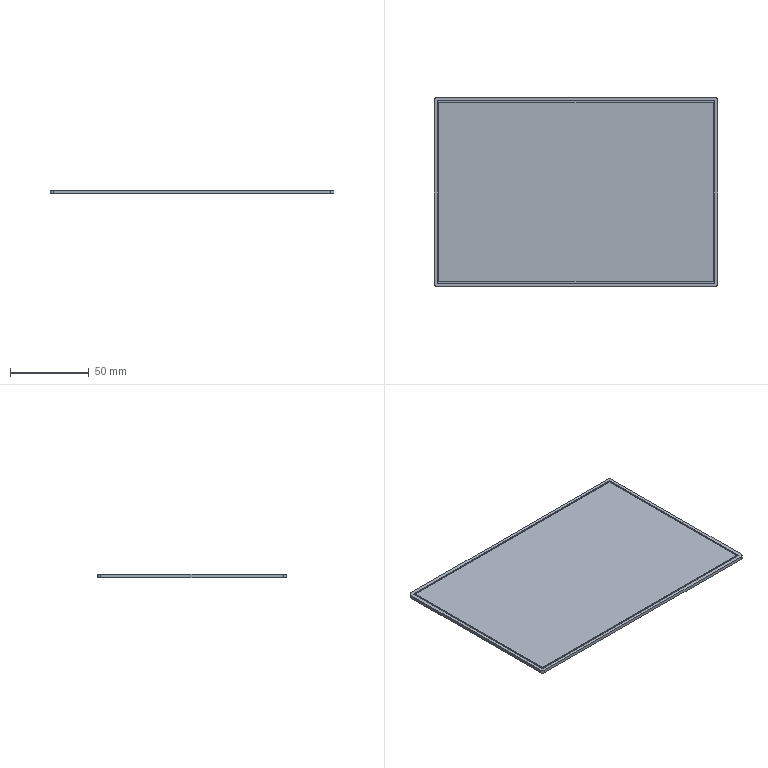Part | SolidWorks | features Extrusion 1, ICE 1 | 1 solid | 20 faces | box 180 x 120 x 2 mm | volume 42903 mm3 | plane 16 | cylinder 4 | commonest cylinder face diameters 4 x4
STEP:
#1=CARTESIAN_POINT('',(90.,58.,0.));
#2=VERTEX_POINT('',#1);
#3=CARTESIAN_POINT('',(88.,60.,0.));
#4=VERTEX_POINT('',#3);
#5=CARTESIAN_POINT('',(88.,58.,0.));
#6=DIRECTION('',(0.,0.,1.));
#7=DIRECTION('',(-1.,0.,0.));
#8=AXIS2_PLACEMENT_3D('',#5,#6,#7);
#9=CIRCLE('',#8,2.);
#10=EDGE_CURVE('',#2,#4,#9,.T.);
#11=ORIENTED_EDGE('',*,*,#10,.T.);
#12=CARTESIAN_POINT('',(88.,60.,2.));
#13=VERTEX_POINT('',#12);
#14=CARTESIAN_POINT('',(88.,60.,2.));
#15=DIRECTION('',(0.,0.,-1.));
#16=VECTOR('',#15,1000.);
#17=LINE('',#14,#16);
#18=EDGE_CURVE('',#13,#4,#17,.T.);
#19=ORIENTED_EDGE('',*,*,#18,.F.);
#20=CARTESIAN_POINT('',(90.,58.,2.));
#21=VERTEX_POINT('',#20);
#22=CARTESIAN_POINT('',(88.,58.,2.));
#23=DIRECTION('',(0.,0.,1.));
#24=DIRECTION('',(-1.,0.,0.));
#25=AXIS2_PLACEMENT_3D('',#22,#23,#24);
#26=CIRCLE('',#25,2.);
#27=EDGE_CURVE('',#21,#13,#26,.T.);
#28=ORIENTED_EDGE('',*,*,#27,.F.);
#29=CARTESIAN_POINT('',(90.,58.,2.));
#30=DIRECTION('',(0.,0.,-1.));
#31=VECTOR('',#30,1000.);
#32=LINE('',#29,#31);
#33=EDGE_CURVE('',#21,#2,#32,.T.);
#34=ORIENTED_EDGE('',*,*,#33,.T.);
#35=EDGE_LOOP('',(#11,#19,#28,#34));
#36=FACE_OUTER_BOUND('',#35,.T.);
#37=CARTESIAN_POINT('',(88.,58.,2.));
#38=DIRECTION('',(0.,0.,-1.));
#39=DIRECTION('',(-1.,0.,0.));
#40=AXIS2_PLACEMENT_3D('',#37,#38,#39);
#41=CYLINDRICAL_SURFACE('',#40,2.);
#42=ADVANCED_FACE('',(#36),#41,.T.);
#43=CARTESIAN_POINT('',(-88.,60.,0.));
#44=VERTEX_POINT('',#43);
#45=CARTESIAN_POINT('',(88.,60.,0.));
#46=DIRECTION('',(-1.,0.,0.));
#47=VECTOR('',#46,1000.);
#48=LINE('',#45,#47);
#49=EDGE_CURVE('',#4,#44,#48,.T.);
#50=ORIENTED_EDGE('',*,*,#49,.T.);
#51=CARTESIAN_POINT('',(-88.,60.,2.));
#52=VERTEX_POINT('',#51);
#53=CARTESIAN_POINT('',(-88.,60.,2.));
#54=DIRECTION('',(0.,0.,-1.));
#55=VECTOR('',#54,1000.);
#56=LINE('',#53,#55);
#57=EDGE_CURVE('',#52,#44,#56,.T.);
#58=ORIENTED_EDGE('',*,*,#57,.F.);
#59=CARTESIAN_POINT('',(88.,60.,2.));
#60=DIRECTION('',(-1.,0.,0.));
#61=VECTOR('',#60,1000.);
#62=LINE('',#59,#61);
#63=EDGE_CURVE('',#13,#52,#62,.T.);
#64=ORIENTED_EDGE('',*,*,#63,.F.);
#65=ORIENTED_EDGE('',*,*,#18,.T.);
#66=EDGE_LOOP('',(#50,#58,#64,#65));
#67=FACE_OUTER_BOUND('',#66,.T.);
#68=CARTESIAN_POINT('',(88.,60.,2.));
#69=DIRECTION('',(0.,-1.,0.));
#70=DIRECTION('',(1.,0.,0.));
#71=AXIS2_PLACEMENT_3D('',#68,#69,#70);
#72=PLANE('',#71);
#73=ADVANCED_FACE('',(#67),#72,.F.);
#74=CARTESIAN_POINT('',(-90.,58.,0.));
#75=VERTEX_POINT('',#74);
#76=CARTESIAN_POINT('',(-88.,58.,0.));
#77=DIRECTION('',(0.,0.,1.));
#78=DIRECTION('',(1.,0.,0.));
#79=AXIS2_PLACEMENT_3D('',#76,#77,#78);
#80=CIRCLE('',#79,2.);
#81=EDGE_CURVE('',#44,#75,#80,.T.);
#82=ORIENTED_EDGE('',*,*,#81,.T.);
#83=CARTESIAN_POINT('',(-90.,58.,2.));
#84=VERTEX_POINT('',#83);
#85=CARTESIAN_POINT('',(-90.,58.,2.));
#86=DIRECTION('',(0.,0.,-1.));
#87=VECTOR('',#86,1000.);
#88=LINE('',#85,#87);
#89=EDGE_CURVE('',#84,#75,#88,.T.);
#90=ORIENTED_EDGE('',*,*,#89,.F.);
#91=CARTESIAN_POINT('',(-88.,58.,2.));
#92=DIRECTION('',(0.,0.,1.));
#93=DIRECTION('',(1.,0.,0.));
#94=AXIS2_PLACEMENT_3D('',#91,#92,#93);
#95=CIRCLE('',#94,2.);
#96=EDGE_CURVE('',#52,#84,#95,.T.);
#97=ORIENTED_EDGE('',*,*,#96,.F.);
#98=ORIENTED_EDGE('',*,*,#57,.T.);
#99=EDGE_LOOP('',(#82,#90,#97,#98));
#100=FACE_OUTER_BOUND('',#99,.T.);
#101=CARTESIAN_POINT('',(-88.,58.,2.));
#102=DIRECTION('',(0.,0.,-1.));
#103=DIRECTION('',(-1.,0.,0.));
#104=AXIS2_PLACEMENT_3D('',#101,#102,#103);
#105=CYLINDRICAL_SURFACE('',#104,2.);
#106=ADVANCED_FACE('',(#100),#105,.T.);
#107=CARTESIAN_POINT('',(-90.,-58.,0.));
#108=VERTEX_POINT('',#107);
#109=CARTESIAN_POINT('',(-90.,58.,0.));
#110=DIRECTION('',(0.,-1.,0.));
#111=VECTOR('',#110,1000.);
#112=LINE('',#109,#111);
#113=EDGE_CURVE('',#75,#108,#112,.T.);
#114=ORIENTED_EDGE('',*,*,#113,.T.);
#115=CARTESIAN_POINT('',(-90.,-58.,2.));
#116=VERTEX_POINT('',#115);
#117=CARTESIAN_POINT('',(-90.,-58.,2.));
#118=DIRECTION('',(0.,0.,-1.));
#119=VECTOR('',#118,1000.);
#120=LINE('',#117,#119);
#121=EDGE_CURVE('',#116,#108,#120,.T.);
#122=ORIENTED_EDGE('',*,*,#121,.F.);
#123=CARTESIAN_POINT('',(-90.,58.,2.));
#124=DIRECTION('',(0.,-1.,0.));
#125=VECTOR('',#124,1000.);
#126=LINE('',#123,#125);
#127=EDGE_CURVE('',#84,#116,#126,.T.);
#128=ORIENTED_EDGE('',*,*,#127,.F.);
#129=ORIENTED_EDGE('',*,*,#89,.T.);
#130=EDGE_LOOP('',(#114,#122,#128,#129));
#131=FACE_OUTER_BOUND('',#130,.T.);
#132=CARTESIAN_POINT('',(-90.,58.,2.));
#133=DIRECTION('',(1.,0.,0.));
#134=DIRECTION('',(0.,1.,0.));
#135=AXIS2_PLACEMENT_3D('',#132,#133,#134);
#136=PLANE('',#135);
#137=ADVANCED_FACE('',(#131),#136,.F.);
#138=CARTESIAN_POINT('',(-88.,-60.,0.));
#139=VERTEX_POINT('',#138);
#140=CARTESIAN_POINT('',(-88.,-58.,0.));
#141=DIRECTION('',(0.,0.,1.));
#142=DIRECTION('',(-1.,0.,0.));
#143=AXIS2_PLACEMENT_3D('',#140,#141,#142);
#144=CIRCLE('',#143,2.);
#145=EDGE_CURVE('',#108,#139,#144,.T.);
#146=ORIENTED_EDGE('',*,*,#145,.T.);
#147=CARTESIAN_POINT('',(-88.,-60.,2.));
#148=VERTEX_POINT('',#147);
#149=CARTESIAN_POINT('',(-88.,-60.,2.));
#150=DIRECTION('',(0.,0.,-1.));
#151=VECTOR('',#150,1000.);
#152=LINE('',#149,#151);
#153=EDGE_CURVE('',#148,#139,#152,.T.);
#154=ORIENTED_EDGE('',*,*,#153,.F.);
#155=CARTESIAN_POINT('',(-88.,-58.,2.));
#156=DIRECTION('',(0.,0.,1.));
#157=DIRECTION('',(-1.,0.,0.));
#158=AXIS2_PLACEMENT_3D('',#155,#156,#157);
#159=CIRCLE('',#158,2.);
#160=EDGE_CURVE('',#116,#148,#159,.T.);
#161=ORIENTED_EDGE('',*,*,#160,.F.);
#162=ORIENTED_EDGE('',*,*,#121,.T.);
#163=EDGE_LOOP('',(#146,#154,#161,#162));
#164=FACE_OUTER_BOUND('',#163,.T.);
#165=CARTESIAN_POINT('',(-88.,-58.,2.));
#166=DIRECTION('',(0.,0.,-1.));
#167=DIRECTION('',(-1.,0.,0.));
#168=AXIS2_PLACEMENT_3D('',#165,#166,#167);
#169=CYLINDRICAL_SURFACE('',#168,2.);
#170=ADVANCED_FACE('',(#164),#169,.T.);
#171=CARTESIAN_POINT('',(88.,-60.,0.));
#172=VERTEX_POINT('',#171);
#173=CARTESIAN_POINT('',(88.,-60.,0.));
#174=DIRECTION('',(1.,0.,0.));
#175=VECTOR('',#174,1000.);
#176=LINE('',#173,#175);
#177=EDGE_CURVE('',#139,#172,#176,.T.);
#178=ORIENTED_EDGE('',*,*,#177,.T.);
#179=CARTESIAN_POINT('',(88.,-60.,2.));
#180=VERTEX_POINT('',#179);
#181=CARTESIAN_POINT('',(88.,-60.,2.));
#182=DIRECTION('',(0.,0.,-1.));
#183=VECTOR('',#182,1000.);
#184=LINE('',#181,#183);
#185=EDGE_CURVE('',#180,#172,#184,.T.);
#186=ORIENTED_EDGE('',*,*,#185,.F.);
#187=CARTESIAN_POINT('',(88.,-60.,2.));
#188=DIRECTION('',(1.,0.,0.));
#189=VECTOR('',#188,1000.);
#190=LINE('',#187,#189);
#191=EDGE_CURVE('',#148,#180,#190,.T.);
#192=ORIENTED_EDGE('',*,*,#191,.F.);
#193=ORIENTED_EDGE('',*,*,#153,.T.);
#194=EDGE_LOOP('',(#178,#186,#192,#193));
#195=FACE_OUTER_BOUND('',#194,.T.);
#196=CARTESIAN_POINT('',(88.,-60.,2.));
#197=DIRECTION('',(0.,1.,0.));
#198=DIRECTION('',(-1.,0.,0.));
#199=AXIS2_PLACEMENT_3D('',#196,#197,#198);
#200=PLANE('',#199);
#201=ADVANCED_FACE('',(#195),#200,.F.);
#202=CARTESIAN_POINT('',(90.,-58.,0.));
#203=VERTEX_POINT('',#202);
#204=CARTESIAN_POINT('',(88.,-58.,0.));
#205=DIRECTION('',(0.,0.,1.));
#206=DIRECTION('',(-1.,0.,0.));
#207=AXIS2_PLACEMENT_3D('',#204,#205,#206);
#208=CIRCLE('',#207,2.);
#209=EDGE_CURVE('',#172,#203,#208,.T.);
#210=ORIENTED_EDGE('',*,*,#209,.T.);
#211=CARTESIAN_POINT('',(90.,-58.,2.));
#212=VERTEX_POINT('',#211);
#213=CARTESIAN_POINT('',(90.,-58.,2.));
#214=DIRECTION('',(0.,0.,-1.));
#215=VECTOR('',#214,1000.);
#216=LINE('',#213,#215);
#217=EDGE_CURVE('',#212,#203,#216,.T.);
#218=ORIENTED_EDGE('',*,*,#217,.F.);
#219=CARTESIAN_POINT('',(88.,-58.,2.));
#220=DIRECTION('',(0.,0.,1.));
#221=DIRECTION('',(-1.,0.,0.));
#222=AXIS2_PLACEMENT_3D('',#219,#220,#221);
#223=CIRCLE('',#222,2.);
#224=EDGE_CURVE('',#180,#212,#223,.T.);
#225=ORIENTED_EDGE('',*,*,#224,.F.);
#226=ORIENTED_EDGE('',*,*,#185,.T.);
#227=EDGE_LOOP('',(#210,#218,#225,#226));
#228=FACE_OUTER_BOUND('',#227,.T.);
#229=CARTESIAN_POINT('',(88.,-58.,2.));
#230=DIRECTION('',(0.,0.,-1.));
#231=DIRECTION('',(-1.,0.,0.));
#232=AXIS2_PLACEMENT_3D('',#229,#230,#231);
#233=CYLINDRICAL_SURFACE('',#232,2.);
#234=ADVANCED_FACE('',(#228),#233,.T.);
#235=CARTESIAN_POINT('',(90.,58.,0.));
#236=DIRECTION('',(0.,1.,0.));
#237=VECTOR('',#236,1000.);
#238=LINE('',#235,#237);
#239=EDGE_CURVE('',#203,#2,#238,.T.);
#240=ORIENTED_EDGE('',*,*,#239,.T.);
#241=ORIENTED_EDGE('',*,*,#33,.F.);
#242=CARTESIAN_POINT('',(90.,58.,2.));
#243=DIRECTION('',(0.,1.,0.));
#244=VECTOR('',#243,1000.);
#245=LINE('',#242,#244);
#246=EDGE_CURVE('',#212,#21,#245,.T.);
#247=ORIENTED_EDGE('',*,*,#246,.F.);
#248=ORIENTED_EDGE('',*,*,#217,.T.);
#249=EDGE_LOOP('',(#240,#241,#247,#248));
#250=FACE_OUTER_BOUND('',#249,.T.);
#251=CARTESIAN_POINT('',(90.,58.,2.));
#252=DIRECTION('',(-1.,0.,0.));
#253=DIRECTION('',(0.,-1.,0.));
#254=AXIS2_PLACEMENT_3D('',#251,#252,#253);
#255=PLANE('',#254);
#256=ADVANCED_FACE('',(#250),#255,.F.);
#257=CARTESIAN_POINT('',(-88.,-58.,2.));
#258=VERTEX_POINT('',#257);
#259=CARTESIAN_POINT('',(88.,-58.,2.));
#260=VERTEX_POINT('',#259);
#261=CARTESIAN_POINT('',(88.,-58.,2.));
#262=DIRECTION('',(1.,0.,0.));
#263=VECTOR('',#262,1000.);
#264=LINE('',#261,#263);
#265=EDGE_CURVE('',#258,#260,#264,.T.);
#266=ORIENTED_EDGE('',*,*,#265,.F.);
#267=CARTESIAN_POINT('',(-88.,58.,2.));
#268=VERTEX_POINT('',#267);
#269=CARTESIAN_POINT('',(-88.,58.,2.));
#270=DIRECTION('',(0.,-1.,0.));
#271=VECTOR('',#270,1000.);
#272=LINE('',#269,#271);
#273=EDGE_CURVE('',#268,#258,#272,.T.);
#274=ORIENTED_EDGE('',*,*,#273,.F.);
#275=CARTESIAN_POINT('',(88.,58.,2.));
#276=VERTEX_POINT('',#275);
#277=CARTESIAN_POINT('',(88.,58.,2.));
#278=DIRECTION('',(-1.,0.,0.));
#279=VECTOR('',#278,1000.);
#280=LINE('',#277,#279);
#281=EDGE_CURVE('',#276,#268,#280,.T.);
#282=ORIENTED_EDGE('',*,*,#281,.F.);
#283=CARTESIAN_POINT('',(88.,58.,2.));
#284=DIRECTION('',(0.,1.,0.));
#285=VECTOR('',#284,1000.);
#286=LINE('',#283,#285);
#287=EDGE_CURVE('',#260,#276,#286,.T.);
#288=ORIENTED_EDGE('',*,*,#287,.F.);
#289=EDGE_LOOP('',(#266,#274,#282,#288));
#290=FACE_BOUND('',#289,.T.);
#291=ORIENTED_EDGE('',*,*,#27,.T.);
#292=ORIENTED_EDGE('',*,*,#63,.T.);
#293=ORIENTED_EDGE('',*,*,#96,.T.);
#294=ORIENTED_EDGE('',*,*,#127,.T.);
#295=ORIENTED_EDGE('',*,*,#160,.T.);
#296=ORIENTED_EDGE('',*,*,#191,.T.);
#297=ORIENTED_EDGE('',*,*,#224,.T.);
#298=ORIENTED_EDGE('',*,*,#246,.T.);
#299=EDGE_LOOP('',(#291,#292,#293,#294,#295,#296,#297,#298));
#300=FACE_OUTER_BOUND('',#299,.T.);
#301=CARTESIAN_POINT('',(88.,58.,2.));
#302=DIRECTION('',(0.,0.,-1.));
#303=DIRECTION('',(-1.,0.,0.));
#304=AXIS2_PLACEMENT_3D('',#301,#302,#303);
#305=PLANE('',#304);
#306=ADVANCED_FACE('',(#290,#300),#305,.F.);
#307=ORIENTED_EDGE('',*,*,#10,.F.);
#308=ORIENTED_EDGE('',*,*,#239,.F.);
#309=ORIENTED_EDGE('',*,*,#209,.F.);
#310=ORIENTED_EDGE('',*,*,#177,.F.);
#311=ORIENTED_EDGE('',*,*,#145,.F.);
#312=ORIENTED_EDGE('',*,*,#113,.F.);
#313=ORIENTED_EDGE('',*,*,#81,.F.);
#314=ORIENTED_EDGE('',*,*,#49,.F.);
#315=EDGE_LOOP('',(#307,#308,#309,#310,#311,#312,#313,#314));
#316=FACE_OUTER_BOUND('',#315,.T.);
#317=CARTESIAN_POINT('',(88.,58.,0.));
#318=DIRECTION('',(0.,0.,-1.));
#319=DIRECTION('',(-1.,0.,0.));
#320=AXIS2_PLACEMENT_3D('',#317,#318,#319);
#321=PLANE('',#320);
#322=ADVANCED_FACE('',(#316),#321,.T.);
#323=ORIENTED_EDGE('',*,*,#273,.T.);
#324=CARTESIAN_POINT('',(-88.,-58.,1.5));
#325=VERTEX_POINT('',#324);
#326=CARTESIAN_POINT('',(-88.,-58.,1.5));
#327=DIRECTION('',(0.,0.,1.));
#328=VECTOR('',#327,1000.);
#329=LINE('',#326,#328);
#330=EDGE_CURVE('',#325,#258,#329,.T.);
#331=ORIENTED_EDGE('',*,*,#330,.F.);
#332=CARTESIAN_POINT('',(-88.,58.,1.5));
#333=VERTEX_POINT('',#332);
#334=CARTESIAN_POINT('',(-88.,58.,1.5));
#335=DIRECTION('',(0.,-1.,0.));
#336=VECTOR('',#335,1000.);
#337=LINE('',#334,#336);
#338=EDGE_CURVE('',#333,#325,#337,.T.);
#339=ORIENTED_EDGE('',*,*,#338,.F.);
#340=CARTESIAN_POINT('',(-88.,58.,1.5));
#341=DIRECTION('',(0.,0.,1.));
#342=VECTOR('',#341,1000.);
#343=LINE('',#340,#342);
#344=EDGE_CURVE('',#333,#268,#343,.T.);
#345=ORIENTED_EDGE('',*,*,#344,.T.);
#346=EDGE_LOOP('',(#323,#331,#339,#345));
#347=FACE_OUTER_BOUND('',#346,.T.);
#348=CARTESIAN_POINT('',(-88.,58.,1.5));
#349=DIRECTION('',(-1.,0.,0.));
#350=DIRECTION('',(0.,0.,1.));
#351=AXIS2_PLACEMENT_3D('',#348,#349,#350);
#352=PLANE('',#351);
#353=ADVANCED_FACE('',(#347),#352,.F.);
#354=ORIENTED_EDGE('',*,*,#281,.T.);
#355=ORIENTED_EDGE('',*,*,#344,.F.);
#356=CARTESIAN_POINT('',(88.,58.,1.5));
#357=VERTEX_POINT('',#356);
#358=CARTESIAN_POINT('',(88.,58.,1.5));
#359=DIRECTION('',(-1.,0.,0.));
#360=VECTOR('',#359,1000.);
#361=LINE('',#358,#360);
#362=EDGE_CURVE('',#357,#333,#361,.T.);
#363=ORIENTED_EDGE('',*,*,#362,.F.);
#364=CARTESIAN_POINT('',(88.,58.,1.5));
#365=DIRECTION('',(0.,0.,1.));
#366=VECTOR('',#365,1000.);
#367=LINE('',#364,#366);
#368=EDGE_CURVE('',#357,#276,#367,.T.);
#369=ORIENTED_EDGE('',*,*,#368,.T.);
#370=EDGE_LOOP('',(#354,#355,#363,#369));
#371=FACE_OUTER_BOUND('',#370,.T.);
#372=CARTESIAN_POINT('',(88.,58.,1.5));
#373=DIRECTION('',(0.,1.,0.));
#374=DIRECTION('',(0.,0.,1.));
#375=AXIS2_PLACEMENT_3D('',#372,#373,#374);
#376=PLANE('',#375);
#377=ADVANCED_FACE('',(#371),#376,.F.);
#378=ORIENTED_EDGE('',*,*,#287,.T.);
#379=ORIENTED_EDGE('',*,*,#368,.F.);
#380=CARTESIAN_POINT('',(88.,-58.,1.5));
#381=VERTEX_POINT('',#380);
#382=CARTESIAN_POINT('',(88.,58.,1.5));
#383=DIRECTION('',(0.,1.,0.));
#384=VECTOR('',#383,1000.);
#385=LINE('',#382,#384);
#386=EDGE_CURVE('',#381,#357,#385,.T.);
#387=ORIENTED_EDGE('',*,*,#386,.F.);
#388=CARTESIAN_POINT('',(88.,-58.,1.5));
#389=DIRECTION('',(0.,0.,1.));
#390=VECTOR('',#389,1000.);
#391=LINE('',#388,#390);
#392=EDGE_CURVE('',#381,#260,#391,.T.);
#393=ORIENTED_EDGE('',*,*,#392,.T.);
#394=EDGE_LOOP('',(#378,#379,#387,#393));
#395=FACE_OUTER_BOUND('',#394,.T.);
#396=CARTESIAN_POINT('',(88.,58.,1.5));
#397=DIRECTION('',(1.,0.,0.));
#398=DIRECTION('',(0.,0.,-1.));
#399=AXIS2_PLACEMENT_3D('',#396,#397,#398);
#400=PLANE('',#399);
#401=ADVANCED_FACE('',(#395),#400,.F.);
#402=ORIENTED_EDGE('',*,*,#265,.T.);
#403=ORIENTED_EDGE('',*,*,#392,.F.);
#404=CARTESIAN_POINT('',(88.,-58.,1.5));
#405=DIRECTION('',(1.,0.,0.));
#406=VECTOR('',#405,1000.);
#407=LINE('',#404,#406);
#408=EDGE_CURVE('',#325,#381,#407,.T.);
#409=ORIENTED_EDGE('',*,*,#408,.F.);
#410=ORIENTED_EDGE('',*,*,#330,.T.);
#411=EDGE_LOOP('',(#402,#403,#409,#410));
#412=FACE_OUTER_BOUND('',#411,.T.);
#413=CARTESIAN_POINT('',(88.,-58.,1.5));
#414=DIRECTION('',(0.,-1.,0.));
#415=DIRECTION('',(0.,0.,-1.));
#416=AXIS2_PLACEMENT_3D('',#413,#414,#415);
#417=PLANE('',#416);
#418=ADVANCED_FACE('',(#412),#417,.F.);
#419=CARTESIAN_POINT('',(87.,-57.,1.5));
#420=VERTEX_POINT('',#419);
#421=CARTESIAN_POINT('',(87.,57.,1.5));
#422=VERTEX_POINT('',#421);
#423=CARTESIAN_POINT('',(87.,57.,1.5));
#424=DIRECTION('',(0.,1.,0.));
#425=VECTOR('',#424,1000.);
#426=LINE('',#423,#425);
#427=EDGE_CURVE('',#420,#422,#426,.T.);
#428=ORIENTED_EDGE('',*,*,#427,.F.);
#429=CARTESIAN_POINT('',(-87.,-57.,1.5));
#430=VERTEX_POINT('',#429);
#431=CARTESIAN_POINT('',(87.,-57.,1.5));
#432=DIRECTION('',(1.,0.,0.));
#433=VECTOR('',#432,1000.);
#434=LINE('',#431,#433);
#435=EDGE_CURVE('',#430,#420,#434,.T.);
#436=ORIENTED_EDGE('',*,*,#435,.F.);
#437=CARTESIAN_POINT('',(-87.,57.,1.5));
#438=VERTEX_POINT('',#437);
#439=CARTESIAN_POINT('',(-87.,57.,1.5));
#440=DIRECTION('',(0.,-1.,0.));
#441=VECTOR('',#440,1000.);
#442=LINE('',#439,#441);
#443=EDGE_CURVE('',#438,#430,#442,.T.);
#444=ORIENTED_EDGE('',*,*,#443,.F.);
#445=CARTESIAN_POINT('',(87.,57.,1.5));
#446=DIRECTION('',(-1.,0.,0.));
#447=VECTOR('',#446,1000.);
#448=LINE('',#445,#447);
#449=EDGE_CURVE('',#422,#438,#448,.T.);
#450=ORIENTED_EDGE('',*,*,#449,.F.);
#451=EDGE_LOOP('',(#428,#436,#444,#450));
#452=FACE_BOUND('',#451,.T.);
#453=ORIENTED_EDGE('',*,*,#338,.T.);
#454=ORIENTED_EDGE('',*,*,#408,.T.);
#455=ORIENTED_EDGE('',*,*,#386,.T.);
#456=ORIENTED_EDGE('',*,*,#362,.T.);
#457=EDGE_LOOP('',(#453,#454,#455,#456));
#458=FACE_OUTER_BOUND('',#457,.T.);
#459=CARTESIAN_POINT('',(0.,0.,1.5));
#460=DIRECTION('',(0.,0.,-1.));
#461=DIRECTION('',(-1.,0.,0.));
#462=AXIS2_PLACEMENT_3D('',#459,#460,#461);
#463=PLANE('',#462);
#464=ADVANCED_FACE('',(#452,#458),#463,.F.);
#465=CARTESIAN_POINT('',(87.,-57.,2.));
#466=VERTEX_POINT('',#465);
#467=CARTESIAN_POINT('',(87.,57.,2.));
#468=VERTEX_POINT('',#467);
#469=CARTESIAN_POINT('',(87.,57.,2.));
#470=DIRECTION('',(0.,1.,0.));
#471=VECTOR('',#470,1000.);
#472=LINE('',#469,#471);
#473=EDGE_CURVE('',#466,#468,#472,.T.);
#474=ORIENTED_EDGE('',*,*,#473,.F.);
#475=CARTESIAN_POINT('',(87.,-57.,1.5));
#476=DIRECTION('',(0.,0.,1.));
#477=VECTOR('',#476,1000.);
#478=LINE('',#475,#477);
#479=EDGE_CURVE('',#420,#466,#478,.T.);
#480=ORIENTED_EDGE('',*,*,#479,.F.);
#481=ORIENTED_EDGE('',*,*,#427,.T.);
#482=CARTESIAN_POINT('',(87.,57.,1.5));
#483=DIRECTION('',(0.,0.,1.));
#484=VECTOR('',#483,1000.);
#485=LINE('',#482,#484);
#486=EDGE_CURVE('',#422,#468,#485,.T.);
#487=ORIENTED_EDGE('',*,*,#486,.T.);
#488=EDGE_LOOP('',(#474,#480,#481,#487));
#489=FACE_OUTER_BOUND('',#488,.T.);
#490=CARTESIAN_POINT('',(87.,57.,1.5));
#491=DIRECTION('',(1.,0.,0.));
#492=DIRECTION('',(0.,0.,-1.));
#493=AXIS2_PLACEMENT_3D('',#490,#491,#492);
#494=PLANE('',#493);
#495=ADVANCED_FACE('',(#489),#494,.T.);
#496=CARTESIAN_POINT('',(-87.,-57.,2.));
#497=VERTEX_POINT('',#496);
#498=CARTESIAN_POINT('',(87.,-57.,2.));
#499=DIRECTION('',(1.,0.,0.));
#500=VECTOR('',#499,1000.);
#501=LINE('',#498,#500);
#502=EDGE_CURVE('',#497,#466,#501,.T.);
#503=ORIENTED_EDGE('',*,*,#502,.F.);
#504=CARTESIAN_POINT('',(-87.,-57.,1.5));
#505=DIRECTION('',(0.,0.,1.));
#506=VECTOR('',#505,1000.);
#507=LINE('',#504,#506);
#508=EDGE_CURVE('',#430,#497,#507,.T.);
#509=ORIENTED_EDGE('',*,*,#508,.F.);
#510=ORIENTED_EDGE('',*,*,#435,.T.);
#511=ORIENTED_EDGE('',*,*,#479,.T.);
#512=EDGE_LOOP('',(#503,#509,#510,#511));
#513=FACE_OUTER_BOUND('',#512,.T.);
#514=CARTESIAN_POINT('',(87.,-57.,1.5));
#515=DIRECTION('',(0.,-1.,0.));
#516=DIRECTION('',(1.,0.,0.));
#517=AXIS2_PLACEMENT_3D('',#514,#515,#516);
#518=PLANE('',#517);
#519=ADVANCED_FACE('',(#513),#518,.T.);
#520=CARTESIAN_POINT('',(-87.,57.,2.));
#521=VERTEX_POINT('',#520);
#522=CARTESIAN_POINT('',(-87.,57.,2.));
#523=DIRECTION('',(0.,-1.,0.));
#524=VECTOR('',#523,1000.);
#525=LINE('',#522,#524);
#526=EDGE_CURVE('',#521,#497,#525,.T.);
#527=ORIENTED_EDGE('',*,*,#526,.F.);
#528=CARTESIAN_POINT('',(-87.,57.,1.5));
#529=DIRECTION('',(0.,0.,1.));
#530=VECTOR('',#529,1000.);
#531=LINE('',#528,#530);
#532=EDGE_CURVE('',#438,#521,#531,.T.);
#533=ORIENTED_EDGE('',*,*,#532,.F.);
#534=ORIENTED_EDGE('',*,*,#443,.T.);
#535=ORIENTED_EDGE('',*,*,#508,.T.);
#536=EDGE_LOOP('',(#527,#533,#534,#535));
#537=FACE_OUTER_BOUND('',#536,.T.);
#538=CARTESIAN_POINT('',(-87.,57.,1.5));
#539=DIRECTION('',(-1.,0.,0.));
#540=DIRECTION('',(0.,0.,1.));
#541=AXIS2_PLACEMENT_3D('',#538,#539,#540);
#542=PLANE('',#541);
#543=ADVANCED_FACE('',(#537),#542,.T.);
#544=CARTESIAN_POINT('',(87.,57.,2.));
#545=DIRECTION('',(-1.,0.,0.));
#546=VECTOR('',#545,1000.);
#547=LINE('',#544,#546);
#548=EDGE_CURVE('',#468,#521,#547,.T.);
#549=ORIENTED_EDGE('',*,*,#548,.F.);
#550=ORIENTED_EDGE('',*,*,#486,.F.);
#551=ORIENTED_EDGE('',*,*,#449,.T.);
#552=ORIENTED_EDGE('',*,*,#532,.T.);
#553=EDGE_LOOP('',(#549,#550,#551,#552));
#554=FACE_OUTER_BOUND('',#553,.T.);
#555=CARTESIAN_POINT('',(87.,57.,1.5));
#556=DIRECTION('',(0.,1.,0.));
#557=DIRECTION('',(0.,0.,1.));
#558=AXIS2_PLACEMENT_3D('',#555,#556,#557);
#559=PLANE('',#558);
#560=ADVANCED_FACE('',(#554),#559,.T.);
#561=ORIENTED_EDGE('',*,*,#473,.T.);
#562=ORIENTED_EDGE('',*,*,#548,.T.);
#563=ORIENTED_EDGE('',*,*,#526,.T.);
#564=ORIENTED_EDGE('',*,*,#502,.T.);
#565=EDGE_LOOP('',(#561,#562,#563,#564));
#566=FACE_OUTER_BOUND('',#565,.T.);
#567=CARTESIAN_POINT('',(88.,58.,2.));
#568=DIRECTION('',(0.,0.,-1.));
#569=DIRECTION('',(-1.,0.,0.));
#570=AXIS2_PLACEMENT_3D('',#567,#568,#569);
#571=PLANE('',#570);
#572=ADVANCED_FACE('',(#566),#571,.F.);
#573=CLOSED_SHELL('',(#42,#73,#106,#137,#170,#201,#234,#256,#306,#322,#353,#377,#401,#418,#464,#495,#519,#543,#560,#572));
#574=MANIFOLD_SOLID_BREP('',#573);
#575=CARTESIAN_POINT('',(0.,0.,0.));
#576=DIRECTION('',(0.,0.,1.));
#577=DIRECTION('',(1.,0.,0.));
#578=AXIS2_PLACEMENT_3D('',#575,#576,#577);
#579=(LENGTH_UNIT()NAMED_UNIT(*)SI_UNIT(.MILLI.,.METRE.));
#580=UNCERTAINTY_MEASURE_WITH_UNIT(LENGTH_MEASURE(0.00001),#579,'','');
#581=(NAMED_UNIT(*)PLANE_ANGLE_UNIT()SI_UNIT($,.RADIAN.));
#582=(NAMED_UNIT(*)SI_UNIT($,.STERADIAN.)SOLID_ANGLE_UNIT());
#583=(GEOMETRIC_REPRESENTATION_CONTEXT(3)GLOBAL_UNCERTAINTY_ASSIGNED_CONTEXT((#580))GLOBAL_UNIT_ASSIGNED_CONTEXT((#579,#581,#582))REPRESENTATION_CONTEXT('',''));
#584=ADVANCED_BREP_SHAPE_REPRESENTATION('',(#574,#578),#583);